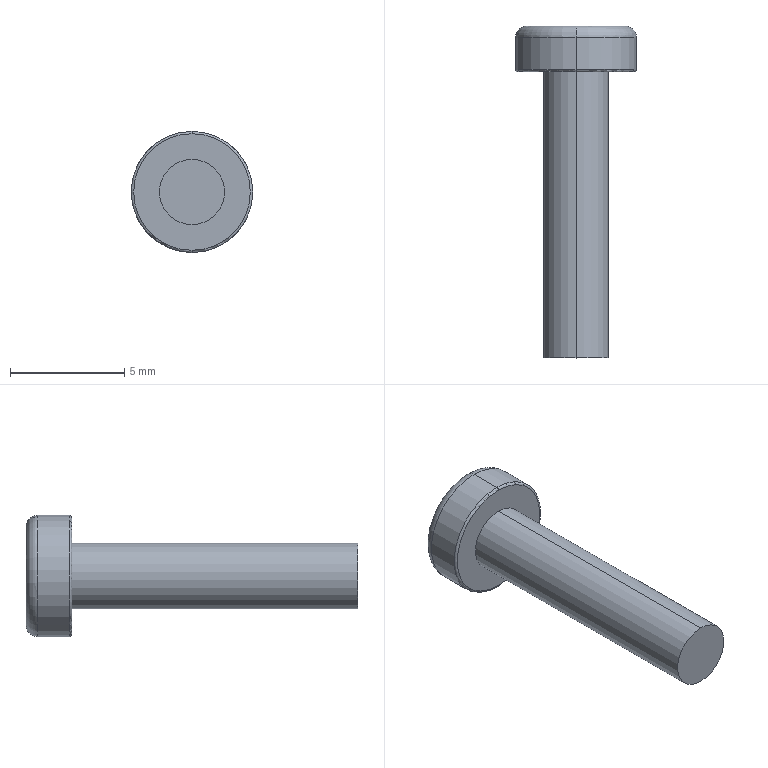Part | SolidWorks | features Fillet 2, ICE 2, Extrusion 1, Helix 1 | 1 solid | 24 faces | box 5.3 x 14.5 x 5.3 mm | volume 122.133 mm3 | plane 16 | torus 4 | cylinder 4 | commonest cylinder face diameters 2.86 x2 5.3 x2
STEP:
#1=CARTESIAN_POINT('',(0.,0.,-2.55));
#2=VERTEX_POINT('',#1);
#3=CARTESIAN_POINT('',(0.,0.,2.55));
#4=VERTEX_POINT('',#3);
#5=CARTESIAN_POINT('',(0.,0.,0.));
#6=DIRECTION('',(0.,-1.,0.));
#7=DIRECTION('',(0.,0.,1.));
#8=AXIS2_PLACEMENT_3D('',#5,#6,#7);
#9=CIRCLE('',#8,2.55);
#10=EDGE_CURVE('',#2,#4,#9,.T.);
#11=ORIENTED_EDGE('',*,*,#10,.F.);
#12=CARTESIAN_POINT('',(0.,0.1,-2.65));
#13=VERTEX_POINT('',#12);
#14=CARTESIAN_POINT('',(0.,0.1,-2.55));
#15=DIRECTION('',(1.,0.,0.));
#16=DIRECTION('',(0.,0.,-1.));
#17=AXIS2_PLACEMENT_3D('',#14,#15,#16);
#18=CIRCLE('',#17,0.1);
#19=EDGE_CURVE('',#2,#13,#18,.T.);
#20=ORIENTED_EDGE('',*,*,#19,.T.);
#21=CARTESIAN_POINT('',(0.,0.1,2.65));
#22=VERTEX_POINT('',#21);
#23=CARTESIAN_POINT('',(0.,0.1,0.));
#24=DIRECTION('',(0.,1.,0.));
#25=DIRECTION('',(0.,0.,1.));
#26=AXIS2_PLACEMENT_3D('',#23,#24,#25);
#27=CIRCLE('',#26,2.65);
#28=EDGE_CURVE('',#22,#13,#27,.T.);
#29=ORIENTED_EDGE('',*,*,#28,.F.);
#30=CARTESIAN_POINT('',(0.,0.1,2.55));
#31=DIRECTION('',(-1.,0.,0.));
#32=DIRECTION('',(0.,0.,1.));
#33=AXIS2_PLACEMENT_3D('',#30,#31,#32);
#34=CIRCLE('',#33,0.1);
#35=EDGE_CURVE('',#4,#22,#34,.T.);
#36=ORIENTED_EDGE('',*,*,#35,.F.);
#37=EDGE_LOOP('',(#11,#20,#29,#36));
#38=FACE_OUTER_BOUND('',#37,.T.);
#39=CARTESIAN_POINT('',(0.,0.1,0.));
#40=DIRECTION('',(0.,1.,0.));
#41=DIRECTION('',(0.,0.,1.));
#42=AXIS2_PLACEMENT_3D('',#39,#40,#41);
#43=TOROIDAL_SURFACE('',#42,2.55,0.1);
#44=ADVANCED_FACE('',(#38),#43,.T.);
#45=CARTESIAN_POINT('',(0.,1.5,-2.65));
#46=VERTEX_POINT('',#45);
#47=CARTESIAN_POINT('',(0.,1.5,2.65));
#48=VERTEX_POINT('',#47);
#49=CARTESIAN_POINT('',(0.,1.5,0.));
#50=DIRECTION('',(0.,-1.,0.));
#51=DIRECTION('',(0.,0.,1.));
#52=AXIS2_PLACEMENT_3D('',#49,#50,#51);
#53=CIRCLE('',#52,2.65);
#54=EDGE_CURVE('',#46,#48,#53,.T.);
#55=ORIENTED_EDGE('',*,*,#54,.F.);
#56=CARTESIAN_POINT('',(0.,2.,-2.15));
#57=VERTEX_POINT('',#56);
#58=CARTESIAN_POINT('',(0.,1.5,-2.15));
#59=DIRECTION('',(1.,0.,0.));
#60=DIRECTION('',(0.,0.,-1.));
#61=AXIS2_PLACEMENT_3D('',#58,#59,#60);
#62=CIRCLE('',#61,0.5);
#63=EDGE_CURVE('',#46,#57,#62,.T.);
#64=ORIENTED_EDGE('',*,*,#63,.T.);
#65=CARTESIAN_POINT('',(0.,2.,2.15));
#66=VERTEX_POINT('',#65);
#67=CARTESIAN_POINT('',(0.,2.,0.));
#68=DIRECTION('',(0.,1.,0.));
#69=DIRECTION('',(0.,0.,1.));
#70=AXIS2_PLACEMENT_3D('',#67,#68,#69);
#71=CIRCLE('',#70,2.15);
#72=EDGE_CURVE('',#66,#57,#71,.T.);
#73=ORIENTED_EDGE('',*,*,#72,.F.);
#74=CARTESIAN_POINT('',(0.,1.5,2.15));
#75=DIRECTION('',(-1.,0.,0.));
#76=DIRECTION('',(0.,0.,1.));
#77=AXIS2_PLACEMENT_3D('',#74,#75,#76);
#78=CIRCLE('',#77,0.5);
#79=EDGE_CURVE('',#48,#66,#78,.T.);
#80=ORIENTED_EDGE('',*,*,#79,.F.);
#81=EDGE_LOOP('',(#55,#64,#73,#80));
#82=FACE_OUTER_BOUND('',#81,.T.);
#83=CARTESIAN_POINT('',(0.,1.5,0.));
#84=DIRECTION('',(0.,1.,0.));
#85=DIRECTION('',(0.,0.,1.));
#86=AXIS2_PLACEMENT_3D('',#83,#84,#85);
#87=TOROIDAL_SURFACE('',#86,2.15,0.5);
#88=ADVANCED_FACE('',(#82),#87,.T.);
#89=CARTESIAN_POINT('',(0.,-12.5,-1.43));
#90=VERTEX_POINT('',#89);
#91=CARTESIAN_POINT('',(0.,-12.5,1.43));
#92=VERTEX_POINT('',#91);
#93=CARTESIAN_POINT('',(0.,-12.5,0.));
#94=DIRECTION('',(0.,-1.,0.));
#95=DIRECTION('',(0.,0.,-1.));
#96=AXIS2_PLACEMENT_3D('',#93,#94,#95);
#97=CIRCLE('',#96,1.43);
#98=EDGE_CURVE('',#90,#92,#97,.T.);
#99=ORIENTED_EDGE('',*,*,#98,.F.);
#100=CARTESIAN_POINT('',(0.,0.,-1.43));
#101=VERTEX_POINT('',#100);
#102=CARTESIAN_POINT('',(0.,-12.5,-1.43));
#103=DIRECTION('',(0.,1.,0.));
#104=VECTOR('',#103,1000.);
#105=LINE('',#102,#104);
#106=EDGE_CURVE('',#90,#101,#105,.T.);
#107=ORIENTED_EDGE('',*,*,#106,.T.);
#108=CARTESIAN_POINT('',(0.,0.,1.43));
#109=VERTEX_POINT('',#108);
#110=CARTESIAN_POINT('',(0.,0.,0.));
#111=DIRECTION('',(0.,-1.,0.));
#112=DIRECTION('',(0.,0.,1.));
#113=AXIS2_PLACEMENT_3D('',#110,#111,#112);
#114=CIRCLE('',#113,1.43);
#115=EDGE_CURVE('',#101,#109,#114,.T.);
#116=ORIENTED_EDGE('',*,*,#115,.T.);
#117=CARTESIAN_POINT('',(0.,-12.5,1.43));
#118=DIRECTION('',(0.,1.,0.));
#119=VECTOR('',#118,1000.);
#120=LINE('',#117,#119);
#121=EDGE_CURVE('',#92,#109,#120,.T.);
#122=ORIENTED_EDGE('',*,*,#121,.F.);
#123=EDGE_LOOP('',(#99,#107,#116,#122));
#124=FACE_OUTER_BOUND('',#123,.T.);
#125=CARTESIAN_POINT('',(0.,-12.5,0.));
#126=DIRECTION('',(0.,1.,0.));
#127=DIRECTION('',(0.,0.,1.));
#128=AXIS2_PLACEMENT_3D('',#125,#126,#127);
#129=CYLINDRICAL_SURFACE('',#128,1.43);
#130=ADVANCED_FACE('',(#124),#129,.T.);
#131=ORIENTED_EDGE('',*,*,#54,.T.);
#132=CARTESIAN_POINT('',(0.,2.,2.65));
#133=DIRECTION('',(0.,-1.,0.));
#134=VECTOR('',#133,1000.);
#135=LINE('',#132,#134);
#136=EDGE_CURVE('',#48,#22,#135,.T.);
#137=ORIENTED_EDGE('',*,*,#136,.T.);
#138=ORIENTED_EDGE('',*,*,#28,.T.);
#139=CARTESIAN_POINT('',(0.,2.,-2.65));
#140=DIRECTION('',(0.,-1.,0.));
#141=VECTOR('',#140,1000.);
#142=LINE('',#139,#141);
#143=EDGE_CURVE('',#46,#13,#142,.T.);
#144=ORIENTED_EDGE('',*,*,#143,.F.);
#145=EDGE_LOOP('',(#131,#137,#138,#144));
#146=FACE_OUTER_BOUND('',#145,.T.);
#147=CARTESIAN_POINT('',(0.,2.,0.));
#148=DIRECTION('',(0.,-1.,0.));
#149=DIRECTION('',(0.,0.,-1.));
#150=AXIS2_PLACEMENT_3D('',#147,#148,#149);
#151=CYLINDRICAL_SURFACE('',#150,2.65);
#152=ADVANCED_FACE('',(#146),#151,.T.);
#153=ORIENTED_EDGE('',*,*,#136,.F.);
#154=CARTESIAN_POINT('',(0.,1.5,0.));
#155=DIRECTION('',(0.,-1.,0.));
#156=DIRECTION('',(0.,0.,1.));
#157=AXIS2_PLACEMENT_3D('',#154,#155,#156);
#158=CIRCLE('',#157,2.65);
#159=EDGE_CURVE('',#48,#46,#158,.T.);
#160=ORIENTED_EDGE('',*,*,#159,.T.);
#161=ORIENTED_EDGE('',*,*,#143,.T.);
#162=CARTESIAN_POINT('',(0.,0.1,0.));
#163=DIRECTION('',(0.,1.,0.));
#164=DIRECTION('',(0.,0.,1.));
#165=AXIS2_PLACEMENT_3D('',#162,#163,#164);
#166=CIRCLE('',#165,2.65);
#167=EDGE_CURVE('',#13,#22,#166,.T.);
#168=ORIENTED_EDGE('',*,*,#167,.T.);
#169=EDGE_LOOP('',(#153,#160,#161,#168));
#170=FACE_OUTER_BOUND('',#169,.T.);
#171=CARTESIAN_POINT('',(0.,2.,0.));
#172=DIRECTION('',(0.,-1.,0.));
#173=DIRECTION('',(0.,0.,-1.));
#174=AXIS2_PLACEMENT_3D('',#171,#172,#173);
#175=CYLINDRICAL_SURFACE('',#174,2.65);
#176=ADVANCED_FACE('',(#170),#175,.T.);
#177=CARTESIAN_POINT('',(1.341,2.,0.3));
#178=VERTEX_POINT('',#177);
#179=CARTESIAN_POINT('',(1.341,2.,-0.3));
#180=VERTEX_POINT('',#179);
#181=CARTESIAN_POINT('',(1.341,2.,0.3));
#182=DIRECTION('',(0.,0.,-1.));
#183=VECTOR('',#182,1000.);
#184=LINE('',#181,#183);
#185=EDGE_CURVE('',#178,#180,#184,.T.);
#186=ORIENTED_EDGE('',*,*,#185,.F.);
#187=CARTESIAN_POINT('',(0.2966,2.,0.3));
#188=VERTEX_POINT('',#187);
#189=CARTESIAN_POINT('',(0.2966,2.,0.3));
#190=DIRECTION('',(1.,0.,0.));
#191=VECTOR('',#190,1000.);
#192=LINE('',#189,#191);
#193=EDGE_CURVE('',#188,#178,#192,.T.);
#194=ORIENTED_EDGE('',*,*,#193,.F.);
#195=CARTESIAN_POINT('',(0.2966,2.,1.336));
#196=VERTEX_POINT('',#195);
#197=CARTESIAN_POINT('',(0.2966,2.,1.336));
#198=DIRECTION('',(0.,0.,-1.));
#199=VECTOR('',#198,1000.);
#200=LINE('',#197,#199);
#201=EDGE_CURVE('',#196,#188,#200,.T.);
#202=ORIENTED_EDGE('',*,*,#201,.F.);
#203=CARTESIAN_POINT('',(-0.3034,2.,1.336));
#204=VERTEX_POINT('',#203);
#205=CARTESIAN_POINT('',(-0.3034,2.,1.336));
#206=DIRECTION('',(1.,0.,0.));
#207=VECTOR('',#206,1000.);
#208=LINE('',#205,#207);
#209=EDGE_CURVE('',#204,#196,#208,.T.);
#210=ORIENTED_EDGE('',*,*,#209,.F.);
#211=CARTESIAN_POINT('',(-0.3034,2.,0.3));
#212=VERTEX_POINT('',#211);
#213=CARTESIAN_POINT('',(-0.3034,2.,1.336));
#214=DIRECTION('',(0.,0.,1.));
#215=VECTOR('',#214,1000.);
#216=LINE('',#213,#215);
#217=EDGE_CURVE('',#212,#204,#216,.T.);
#218=ORIENTED_EDGE('',*,*,#217,.F.);
#219=CARTESIAN_POINT('',(-1.341,2.,0.3));
#220=VERTEX_POINT('',#219);
#221=CARTESIAN_POINT('',(-1.341,2.,0.3));
#222=DIRECTION('',(1.,0.,0.));
#223=VECTOR('',#222,1000.);
#224=LINE('',#221,#223);
#225=EDGE_CURVE('',#220,#212,#224,.T.);
#226=ORIENTED_EDGE('',*,*,#225,.F.);
#227=CARTESIAN_POINT('',(-1.341,2.,-0.3));
#228=VERTEX_POINT('',#227);
#229=CARTESIAN_POINT('',(-1.341,2.,0.3));
#230=DIRECTION('',(0.,0.,1.));
#231=VECTOR('',#230,1000.);
#232=LINE('',#229,#231);
#233=EDGE_CURVE('',#228,#220,#232,.T.);
#234=ORIENTED_EDGE('',*,*,#233,.F.);
#235=CARTESIAN_POINT('',(-0.3034,2.,-0.3));
#236=VERTEX_POINT('',#235);
#237=CARTESIAN_POINT('',(-1.341,2.,-0.3));
#238=DIRECTION('',(-1.,0.,0.));
#239=VECTOR('',#238,1000.);
#240=LINE('',#237,#239);
#241=EDGE_CURVE('',#236,#228,#240,.T.);
#242=ORIENTED_EDGE('',*,*,#241,.F.);
#243=CARTESIAN_POINT('',(-0.3034,2.,-1.336));
#244=VERTEX_POINT('',#243);
#245=CARTESIAN_POINT('',(-0.3034,2.,-0.3));
#246=DIRECTION('',(0.,0.,1.));
#247=VECTOR('',#246,1000.);
#248=LINE('',#245,#247);
#249=EDGE_CURVE('',#244,#236,#248,.T.);
#250=ORIENTED_EDGE('',*,*,#249,.F.);
#251=CARTESIAN_POINT('',(0.2966,2.,-1.336));
#252=VERTEX_POINT('',#251);
#253=CARTESIAN_POINT('',(-0.3034,2.,-1.336));
#254=DIRECTION('',(-1.,0.,0.));
#255=VECTOR('',#254,1000.);
#256=LINE('',#253,#255);
#257=EDGE_CURVE('',#252,#244,#256,.T.);
#258=ORIENTED_EDGE('',*,*,#257,.F.);
#259=CARTESIAN_POINT('',(0.2966,2.,-0.3));
#260=VERTEX_POINT('',#259);
#261=CARTESIAN_POINT('',(0.2966,2.,-0.3));
#262=DIRECTION('',(0.,0.,-1.));
#263=VECTOR('',#262,1000.);
#264=LINE('',#261,#263);
#265=EDGE_CURVE('',#260,#252,#264,.T.);
#266=ORIENTED_EDGE('',*,*,#265,.F.);
#267=CARTESIAN_POINT('',(0.2966,2.,-0.3));
#268=DIRECTION('',(-1.,0.,0.));
#269=VECTOR('',#268,1000.);
#270=LINE('',#267,#269);
#271=EDGE_CURVE('',#180,#260,#270,.T.);
#272=ORIENTED_EDGE('',*,*,#271,.F.);
#273=EDGE_LOOP('',(#186,#194,#202,#210,#218,#226,#234,#242,#250,#258,#266,#272));
#274=FACE_BOUND('',#273,.T.);
#275=ORIENTED_EDGE('',*,*,#72,.T.);
#276=CARTESIAN_POINT('',(0.,2.,0.));
#277=DIRECTION('',(0.,1.,0.));
#278=DIRECTION('',(0.,0.,1.));
#279=AXIS2_PLACEMENT_3D('',#276,#277,#278);
#280=CIRCLE('',#279,2.15);
#281=EDGE_CURVE('',#57,#66,#280,.T.);
#282=ORIENTED_EDGE('',*,*,#281,.T.);
#283=EDGE_LOOP('',(#275,#282));
#284=FACE_OUTER_BOUND('',#283,.T.);
#285=CARTESIAN_POINT('',(0.,2.,0.));
#286=DIRECTION('',(0.,1.,0.));
#287=DIRECTION('',(0.,0.,1.));
#288=AXIS2_PLACEMENT_3D('',#285,#286,#287);
#289=PLANE('',#288);
#290=ADVANCED_FACE('',(#274,#284),#289,.T.);
#291=CARTESIAN_POINT('',(0.,0.,0.));
#292=DIRECTION('',(0.,-1.,0.));
#293=DIRECTION('',(0.,0.,1.));
#294=AXIS2_PLACEMENT_3D('',#291,#292,#293);
#295=CIRCLE('',#294,2.55);
#296=EDGE_CURVE('',#4,#2,#295,.T.);
#297=ORIENTED_EDGE('',*,*,#296,.T.);
#298=ORIENTED_EDGE('',*,*,#10,.T.);
#299=EDGE_LOOP('',(#297,#298));
#300=FACE_OUTER_BOUND('',#299,.T.);
#301=CARTESIAN_POINT('',(0.,0.,0.));
#302=DIRECTION('',(0.,-1.,0.));
#303=DIRECTION('',(0.,0.,1.));
#304=AXIS2_PLACEMENT_3D('',#301,#302,#303);
#305=CIRCLE('',#304,1.43);
#306=EDGE_CURVE('',#109,#101,#305,.T.);
#307=ORIENTED_EDGE('',*,*,#306,.F.);
#308=ORIENTED_EDGE('',*,*,#115,.F.);
#309=EDGE_LOOP('',(#307,#308));
#310=FACE_BOUND('',#309,.T.);
#311=CARTESIAN_POINT('',(0.,0.,0.));
#312=DIRECTION('',(0.,1.,0.));
#313=DIRECTION('',(0.,0.,1.));
#314=AXIS2_PLACEMENT_3D('',#311,#312,#313);
#315=PLANE('',#314);
#316=ADVANCED_FACE('',(#300,#310),#315,.F.);
#317=ORIENTED_EDGE('',*,*,#106,.F.);
#318=CARTESIAN_POINT('',(0.,-12.5,0.));
#319=DIRECTION('',(0.,-1.,0.));
#320=DIRECTION('',(0.,0.,-1.));
#321=AXIS2_PLACEMENT_3D('',#318,#319,#320);
#322=CIRCLE('',#321,1.43);
#323=EDGE_CURVE('',#92,#90,#322,.T.);
#324=ORIENTED_EDGE('',*,*,#323,.F.);
#325=ORIENTED_EDGE('',*,*,#121,.T.);
#326=ORIENTED_EDGE('',*,*,#306,.T.);
#327=EDGE_LOOP('',(#317,#324,#325,#326));
#328=FACE_OUTER_BOUND('',#327,.T.);
#329=CARTESIAN_POINT('',(0.,-12.5,0.));
#330=DIRECTION('',(0.,1.,0.));
#331=DIRECTION('',(0.,0.,1.));
#332=AXIS2_PLACEMENT_3D('',#329,#330,#331);
#333=CYLINDRICAL_SURFACE('',#332,1.43);
#334=ADVANCED_FACE('',(#328),#333,.T.);
#335=ORIENTED_EDGE('',*,*,#323,.T.);
#336=ORIENTED_EDGE('',*,*,#98,.T.);
#337=EDGE_LOOP('',(#335,#336));
#338=FACE_OUTER_BOUND('',#337,.T.);
#339=CARTESIAN_POINT('',(0.,-12.5,0.));
#340=DIRECTION('',(0.,-1.,0.));
#341=DIRECTION('',(0.,0.,-1.));
#342=AXIS2_PLACEMENT_3D('',#339,#340,#341);
#343=PLANE('',#342);
#344=ADVANCED_FACE('',(#338),#343,.T.);
#345=ORIENTED_EDGE('',*,*,#63,.F.);
#346=ORIENTED_EDGE('',*,*,#159,.F.);
#347=ORIENTED_EDGE('',*,*,#79,.T.);
#348=ORIENTED_EDGE('',*,*,#281,.F.);
#349=EDGE_LOOP('',(#345,#346,#347,#348));
#350=FACE_OUTER_BOUND('',#349,.T.);
#351=CARTESIAN_POINT('',(0.,1.5,0.));
#352=DIRECTION('',(0.,1.,0.));
#353=DIRECTION('',(0.,0.,1.));
#354=AXIS2_PLACEMENT_3D('',#351,#352,#353);
#355=TOROIDAL_SURFACE('',#354,2.15,0.5);
#356=ADVANCED_FACE('',(#350),#355,.T.);
#357=ORIENTED_EDGE('',*,*,#19,.F.);
#358=ORIENTED_EDGE('',*,*,#296,.F.);
#359=ORIENTED_EDGE('',*,*,#35,.T.);
#360=ORIENTED_EDGE('',*,*,#167,.F.);
#361=EDGE_LOOP('',(#357,#358,#359,#360));
#362=FACE_OUTER_BOUND('',#361,.T.);
#363=CARTESIAN_POINT('',(0.,0.1,0.));
#364=DIRECTION('',(0.,1.,0.));
#365=DIRECTION('',(0.,0.,1.));
#366=AXIS2_PLACEMENT_3D('',#363,#364,#365);
#367=TOROIDAL_SURFACE('',#366,2.55,0.1);
#368=ADVANCED_FACE('',(#362),#367,.T.);
#369=ORIENTED_EDGE('',*,*,#185,.T.);
#370=CARTESIAN_POINT('',(1.332,1.5,-0.2913));
#371=VERTEX_POINT('',#370);
#372=CARTESIAN_POINT('',(1.34,1.99,-0.2998));
#373=DIRECTION('',(0.01745,0.9997,-0.01745));
#374=VECTOR('',#373,1000.);
#375=LINE('',#372,#374);
#376=EDGE_CURVE('',#371,#180,#375,.T.);
#377=ORIENTED_EDGE('',*,*,#376,.F.);
#378=CARTESIAN_POINT('',(1.332,1.5,0.2913));
#379=VERTEX_POINT('',#378);
#380=CARTESIAN_POINT('',(1.332,1.5,0.3));
#381=DIRECTION('',(0.,0.,-1.));
#382=VECTOR('',#381,1000.);
#383=LINE('',#380,#382);
#384=EDGE_CURVE('',#379,#371,#383,.T.);
#385=ORIENTED_EDGE('',*,*,#384,.F.);
#386=CARTESIAN_POINT('',(1.34,1.982,0.2997));
#387=DIRECTION('',(0.01745,0.9997,0.01745));
#388=VECTOR('',#387,1000.);
#389=LINE('',#386,#388);
#390=EDGE_CURVE('',#379,#178,#389,.T.);
#391=ORIENTED_EDGE('',*,*,#390,.T.);
#392=EDGE_LOOP('',(#369,#377,#385,#391));
#393=FACE_OUTER_BOUND('',#392,.T.);
#394=CARTESIAN_POINT('',(1.341,2.,0.3));
#395=DIRECTION('',(0.9998,-0.01745,0.));
#396=DIRECTION('',(0.01745,0.9998,0.));
#397=AXIS2_PLACEMENT_3D('',#394,#395,#396);
#398=PLANE('',#397);
#399=ADVANCED_FACE('',(#393),#398,.F.);
#400=ORIENTED_EDGE('',*,*,#193,.T.);
#401=ORIENTED_EDGE('',*,*,#390,.F.);
#402=CARTESIAN_POINT('',(0.2878,1.5,0.2913));
#403=VERTEX_POINT('',#402);
#404=CARTESIAN_POINT('',(0.2966,1.5,0.2913));
#405=DIRECTION('',(1.,0.,0.));
#406=VECTOR('',#405,1000.);
#407=LINE('',#404,#406);
#408=EDGE_CURVE('',#403,#379,#407,.T.);
#409=ORIENTED_EDGE('',*,*,#408,.F.);
#410=CARTESIAN_POINT('',(0.2966,2.,0.3));
#411=DIRECTION('',(0.01745,0.9997,0.01745));
#412=VECTOR('',#411,1000.);
#413=LINE('',#410,#412);
#414=EDGE_CURVE('',#403,#188,#413,.T.);
#415=ORIENTED_EDGE('',*,*,#414,.T.);
#416=EDGE_LOOP('',(#400,#401,#409,#415));
#417=FACE_OUTER_BOUND('',#416,.T.);
#418=CARTESIAN_POINT('',(0.2966,2.,0.3));
#419=DIRECTION('',(0.,-0.01745,0.9998));
#420=DIRECTION('',(0.,-0.9998,-0.01745));
#421=AXIS2_PLACEMENT_3D('',#418,#419,#420);
#422=PLANE('',#421);
#423=ADVANCED_FACE('',(#417),#422,.F.);
#424=ORIENTED_EDGE('',*,*,#201,.T.);
#425=ORIENTED_EDGE('',*,*,#414,.F.);
#426=CARTESIAN_POINT('',(0.2878,1.5,1.327));
#427=VERTEX_POINT('',#426);
#428=CARTESIAN_POINT('',(0.2878,1.5,1.336));
#429=DIRECTION('',(0.,0.,-1.));
#430=VECTOR('',#429,1000.);
#431=LINE('',#428,#430);
#432=EDGE_CURVE('',#427,#403,#431,.T.);
#433=ORIENTED_EDGE('',*,*,#432,.F.);
#434=CARTESIAN_POINT('',(0.2964,1.99,1.336));
#435=DIRECTION('',(0.01745,0.9997,0.01745));
#436=VECTOR('',#435,1000.);
#437=LINE('',#434,#436);
#438=EDGE_CURVE('',#427,#196,#437,.T.);
#439=ORIENTED_EDGE('',*,*,#438,.T.);
#440=EDGE_LOOP('',(#424,#425,#433,#439));
#441=FACE_OUTER_BOUND('',#440,.T.);
#442=CARTESIAN_POINT('',(0.2966,2.,1.336));
#443=DIRECTION('',(0.9998,-0.01745,0.));
#444=DIRECTION('',(0.01745,0.9998,0.));
#445=AXIS2_PLACEMENT_3D('',#442,#443,#444);
#446=PLANE('',#445);
#447=ADVANCED_FACE('',(#441),#446,.F.);
#448=ORIENTED_EDGE('',*,*,#209,.T.);
#449=ORIENTED_EDGE('',*,*,#438,.F.);
#450=CARTESIAN_POINT('',(-0.2947,1.5,1.327));
#451=VERTEX_POINT('',#450);
#452=CARTESIAN_POINT('',(-0.3034,1.5,1.327));
#453=DIRECTION('',(1.,0.,0.));
#454=VECTOR('',#453,1000.);
#455=LINE('',#452,#454);
#456=EDGE_CURVE('',#451,#427,#455,.T.);
#457=ORIENTED_EDGE('',*,*,#456,.F.);
#458=CARTESIAN_POINT('',(-0.3034,2.,1.336));
#459=DIRECTION('',(-0.01745,0.9997,0.01745));
#460=VECTOR('',#459,1000.);
#461=LINE('',#458,#460);
#462=EDGE_CURVE('',#451,#204,#461,.T.);
#463=ORIENTED_EDGE('',*,*,#462,.T.);
#464=EDGE_LOOP('',(#448,#449,#457,#463));
#465=FACE_OUTER_BOUND('',#464,.T.);
#466=CARTESIAN_POINT('',(-0.3034,2.,1.336));
#467=DIRECTION('',(0.,-0.01745,0.9998));
#468=DIRECTION('',(0.,-0.9998,-0.01745));
#469=AXIS2_PLACEMENT_3D('',#466,#467,#468);
#470=PLANE('',#469);
#471=ADVANCED_FACE('',(#465),#470,.F.);
#472=ORIENTED_EDGE('',*,*,#217,.T.);
#473=ORIENTED_EDGE('',*,*,#462,.F.);
#474=CARTESIAN_POINT('',(-0.2947,1.5,0.2913));
#475=VERTEX_POINT('',#474);
#476=CARTESIAN_POINT('',(-0.2947,1.5,1.336));
#477=DIRECTION('',(0.,0.,1.));
#478=VECTOR('',#477,1000.);
#479=LINE('',#476,#478);
#480=EDGE_CURVE('',#475,#451,#479,.T.);
#481=ORIENTED_EDGE('',*,*,#480,.F.);
#482=CARTESIAN_POINT('',(-0.3037,2.018,0.3003));
#483=DIRECTION('',(-0.01745,0.9997,0.01745));
#484=VECTOR('',#483,1000.);
#485=LINE('',#482,#484);
#486=EDGE_CURVE('',#475,#212,#485,.T.);
#487=ORIENTED_EDGE('',*,*,#486,.T.);
#488=EDGE_LOOP('',(#472,#473,#481,#487));
#489=FACE_OUTER_BOUND('',#488,.T.);
#490=CARTESIAN_POINT('',(-0.3034,2.,1.336));
#491=DIRECTION('',(-0.9998,-0.01745,0.));
#492=DIRECTION('',(0.01745,-0.9998,0.));
#493=AXIS2_PLACEMENT_3D('',#490,#491,#492);
#494=PLANE('',#493);
#495=ADVANCED_FACE('',(#489),#494,.F.);
#496=ORIENTED_EDGE('',*,*,#225,.T.);
#497=ORIENTED_EDGE('',*,*,#486,.F.);
#498=CARTESIAN_POINT('',(-1.332,1.5,0.2913));
#499=VERTEX_POINT('',#498);
#500=CARTESIAN_POINT('',(-1.341,1.5,0.2913));
#501=DIRECTION('',(1.,0.,0.));
#502=VECTOR('',#501,1000.);
#503=LINE('',#500,#502);
#504=EDGE_CURVE('',#499,#475,#503,.T.);
#505=ORIENTED_EDGE('',*,*,#504,.F.);
#506=CARTESIAN_POINT('',(-1.341,2.,0.3));
#507=DIRECTION('',(-0.01745,0.9997,0.01745));
#508=VECTOR('',#507,1000.);
#509=LINE('',#506,#508);
#510=EDGE_CURVE('',#499,#220,#509,.T.);
#511=ORIENTED_EDGE('',*,*,#510,.T.);
#512=EDGE_LOOP('',(#496,#497,#505,#511));
#513=FACE_OUTER_BOUND('',#512,.T.);
#514=CARTESIAN_POINT('',(-1.341,2.,0.3));
#515=DIRECTION('',(0.,-0.01745,0.9998));
#516=DIRECTION('',(0.,-0.9998,-0.01745));
#517=AXIS2_PLACEMENT_3D('',#514,#515,#516);
#518=PLANE('',#517);
#519=ADVANCED_FACE('',(#513),#518,.F.);
#520=ORIENTED_EDGE('',*,*,#233,.T.);
#521=ORIENTED_EDGE('',*,*,#510,.F.);
#522=CARTESIAN_POINT('',(-1.332,1.5,-0.2913));
#523=VERTEX_POINT('',#522);
#524=CARTESIAN_POINT('',(-1.332,1.5,0.3));
#525=DIRECTION('',(0.,0.,1.));
#526=VECTOR('',#525,1000.);
#527=LINE('',#524,#526);
#528=EDGE_CURVE('',#523,#499,#527,.T.);
#529=ORIENTED_EDGE('',*,*,#528,.F.);
#530=CARTESIAN_POINT('',(-1.341,2.,-0.3));
#531=DIRECTION('',(-0.01745,0.9997,-0.01745));
#532=VECTOR('',#531,1000.);
#533=LINE('',#530,#532);
#534=EDGE_CURVE('',#523,#228,#533,.T.);
#535=ORIENTED_EDGE('',*,*,#534,.T.);
#536=EDGE_LOOP('',(#520,#521,#529,#535));
#537=FACE_OUTER_BOUND('',#536,.T.);
#538=CARTESIAN_POINT('',(-1.341,2.,0.3));
#539=DIRECTION('',(-0.9998,-0.01745,0.));
#540=DIRECTION('',(0.01745,-0.9998,0.));
#541=AXIS2_PLACEMENT_3D('',#538,#539,#540);
#542=PLANE('',#541);
#543=ADVANCED_FACE('',(#537),#542,.F.);
#544=ORIENTED_EDGE('',*,*,#241,.T.);
#545=ORIENTED_EDGE('',*,*,#534,.F.);
#546=CARTESIAN_POINT('',(-0.2947,1.5,-0.2913));
#547=VERTEX_POINT('',#546);
#548=CARTESIAN_POINT('',(-1.341,1.5,-0.2913));
#549=DIRECTION('',(-1.,0.,0.));
#550=VECTOR('',#549,1000.);
#551=LINE('',#548,#550);
#552=EDGE_CURVE('',#547,#523,#551,.T.);
#553=ORIENTED_EDGE('',*,*,#552,.F.);
#554=CARTESIAN_POINT('',(-0.3037,2.018,-0.3003));
#555=DIRECTION('',(-0.01745,0.9997,-0.01745));
#556=VECTOR('',#555,1000.);
#557=LINE('',#554,#556);
#558=EDGE_CURVE('',#547,#236,#557,.T.);
#559=ORIENTED_EDGE('',*,*,#558,.T.);
#560=EDGE_LOOP('',(#544,#545,#553,#559));
#561=FACE_OUTER_BOUND('',#560,.T.);
#562=CARTESIAN_POINT('',(-1.341,2.,-0.3));
#563=DIRECTION('',(0.,-0.01745,-0.9998));
#564=DIRECTION('',(0.,0.9998,-0.01745));
#565=AXIS2_PLACEMENT_3D('',#562,#563,#564);
#566=PLANE('',#565);
#567=ADVANCED_FACE('',(#561),#566,.F.);
#568=ORIENTED_EDGE('',*,*,#249,.T.);
#569=ORIENTED_EDGE('',*,*,#558,.F.);
#570=CARTESIAN_POINT('',(-0.2947,1.5,-1.327));
#571=VERTEX_POINT('',#570);
#572=CARTESIAN_POINT('',(-0.2947,1.5,-0.3));
#573=DIRECTION('',(0.,0.,1.));
#574=VECTOR('',#573,1000.);
#575=LINE('',#572,#574);
#576=EDGE_CURVE('',#571,#547,#575,.T.);
#577=ORIENTED_EDGE('',*,*,#576,.F.);
#578=CARTESIAN_POINT('',(-0.3034,2.,-1.336));
#579=DIRECTION('',(-0.01745,0.9997,-0.01745));
#580=VECTOR('',#579,1000.);
#581=LINE('',#578,#580);
#582=EDGE_CURVE('',#571,#244,#581,.T.);
#583=ORIENTED_EDGE('',*,*,#582,.T.);
#584=EDGE_LOOP('',(#568,#569,#577,#583));
#585=FACE_OUTER_BOUND('',#584,.T.);
#586=CARTESIAN_POINT('',(-0.3034,2.,-0.3));
#587=DIRECTION('',(-0.9998,-0.01745,0.));
#588=DIRECTION('',(0.01745,-0.9998,0.));
#589=AXIS2_PLACEMENT_3D('',#586,#587,#588);
#590=PLANE('',#589);
#591=ADVANCED_FACE('',(#585),#590,.F.);
#592=ORIENTED_EDGE('',*,*,#257,.T.);
#593=ORIENTED_EDGE('',*,*,#582,.F.);
#594=CARTESIAN_POINT('',(0.2878,1.5,-1.327));
#595=VERTEX_POINT('',#594);
#596=CARTESIAN_POINT('',(-0.3034,1.5,-1.327));
#597=DIRECTION('',(-1.,0.,0.));
#598=VECTOR('',#597,1000.);
#599=LINE('',#596,#598);
#600=EDGE_CURVE('',#595,#571,#599,.T.);
#601=ORIENTED_EDGE('',*,*,#600,.F.);
#602=CARTESIAN_POINT('',(0.2963,1.982,-1.336));
#603=DIRECTION('',(0.01745,0.9997,-0.01745));
#604=VECTOR('',#603,1000.);
#605=LINE('',#602,#604);
#606=EDGE_CURVE('',#595,#252,#605,.T.);
#607=ORIENTED_EDGE('',*,*,#606,.T.);
#608=EDGE_LOOP('',(#592,#593,#601,#607));
#609=FACE_OUTER_BOUND('',#608,.T.);
#610=CARTESIAN_POINT('',(-0.3034,2.,-1.336));
#611=DIRECTION('',(0.,-0.01745,-0.9998));
#612=DIRECTION('',(0.,0.9998,-0.01745));
#613=AXIS2_PLACEMENT_3D('',#610,#611,#612);
#614=PLANE('',#613);
#615=ADVANCED_FACE('',(#609),#614,.F.);
#616=ORIENTED_EDGE('',*,*,#265,.T.);
#617=ORIENTED_EDGE('',*,*,#606,.F.);
#618=CARTESIAN_POINT('',(0.2878,1.5,-0.2913));
#619=VERTEX_POINT('',#618);
#620=CARTESIAN_POINT('',(0.2878,1.5,-0.3));
#621=DIRECTION('',(0.,0.,-1.));
#622=VECTOR('',#621,1000.);
#623=LINE('',#620,#622);
#624=EDGE_CURVE('',#619,#595,#623,.T.);
#625=ORIENTED_EDGE('',*,*,#624,.F.);
#626=CARTESIAN_POINT('',(0.2966,2.,-0.3));
#627=DIRECTION('',(0.01745,0.9997,-0.01745));
#628=VECTOR('',#627,1000.);
#629=LINE('',#626,#628);
#630=EDGE_CURVE('',#619,#260,#629,.T.);
#631=ORIENTED_EDGE('',*,*,#630,.T.);
#632=EDGE_LOOP('',(#616,#617,#625,#631));
#633=FACE_OUTER_BOUND('',#632,.T.);
#634=CARTESIAN_POINT('',(0.2966,2.,-0.3));
#635=DIRECTION('',(0.9998,-0.01745,0.));
#636=DIRECTION('',(0.01745,0.9998,0.));
#637=AXIS2_PLACEMENT_3D('',#634,#635,#636);
#638=PLANE('',#637);
#639=ADVANCED_FACE('',(#633),#638,.F.);
#640=ORIENTED_EDGE('',*,*,#271,.T.);
#641=ORIENTED_EDGE('',*,*,#630,.F.);
#642=CARTESIAN_POINT('',(0.2966,1.5,-0.2913));
#643=DIRECTION('',(-1.,0.,0.));
#644=VECTOR('',#643,1000.);
#645=LINE('',#642,#644);
#646=EDGE_CURVE('',#371,#619,#645,.T.);
#647=ORIENTED_EDGE('',*,*,#646,.F.);
#648=ORIENTED_EDGE('',*,*,#376,.T.);
#649=EDGE_LOOP('',(#640,#641,#647,#648));
#650=FACE_OUTER_BOUND('',#649,.T.);
#651=CARTESIAN_POINT('',(0.2966,2.,-0.3));
#652=DIRECTION('',(0.,-0.01745,-0.9998));
#653=DIRECTION('',(0.,0.9998,-0.01745));
#654=AXIS2_PLACEMENT_3D('',#651,#652,#653);
#655=PLANE('',#654);
#656=ADVANCED_FACE('',(#650),#655,.F.);
#657=ORIENTED_EDGE('',*,*,#384,.T.);
#658=ORIENTED_EDGE('',*,*,#646,.T.);
#659=ORIENTED_EDGE('',*,*,#624,.T.);
#660=ORIENTED_EDGE('',*,*,#600,.T.);
#661=ORIENTED_EDGE('',*,*,#576,.T.);
#662=ORIENTED_EDGE('',*,*,#552,.T.);
#663=ORIENTED_EDGE('',*,*,#528,.T.);
#664=ORIENTED_EDGE('',*,*,#504,.T.);
#665=ORIENTED_EDGE('',*,*,#480,.T.);
#666=ORIENTED_EDGE('',*,*,#456,.T.);
#667=ORIENTED_EDGE('',*,*,#432,.T.);
#668=ORIENTED_EDGE('',*,*,#408,.T.);
#669=EDGE_LOOP('',(#657,#658,#659,#660,#661,#662,#663,#664,#665,#666,#667,#668));
#670=FACE_OUTER_BOUND('',#669,.T.);
#671=CARTESIAN_POINT('',(0.,1.5,0.));
#672=DIRECTION('',(0.,-1.,0.));
#673=DIRECTION('',(0.,0.,-1.));
#674=AXIS2_PLACEMENT_3D('',#671,#672,#673);
#675=PLANE('',#674);
#676=ADVANCED_FACE('',(#670),#675,.F.);
#677=CLOSED_SHELL('',(#44,#88,#130,#152,#176,#290,#316,#334,#344,#356,#368,#399,#423,#447,#471,#495,#519,#543,#567,#591,#615,#639,#656,#676));
#678=MANIFOLD_SOLID_BREP('',#677);
#679=CARTESIAN_POINT('',(0.,0.,0.));
#680=DIRECTION('',(0.,0.,1.));
#681=DIRECTION('',(1.,0.,0.));
#682=AXIS2_PLACEMENT_3D('',#679,#680,#681);
#683=(LENGTH_UNIT()NAMED_UNIT(*)SI_UNIT(.MILLI.,.METRE.));
#684=UNCERTAINTY_MEASURE_WITH_UNIT(LENGTH_MEASURE(0.00001),#683,'','');
#685=(NAMED_UNIT(*)PLANE_ANGLE_UNIT()SI_UNIT($,.RADIAN.));
#686=(NAMED_UNIT(*)SI_UNIT($,.STERADIAN.)SOLID_ANGLE_UNIT());
#687=(GEOMETRIC_REPRESENTATION_CONTEXT(3)GLOBAL_UNCERTAINTY_ASSIGNED_CONTEXT((#684))GLOBAL_UNIT_ASSIGNED_CONTEXT((#683,#685,#686))REPRESENTATION_CONTEXT('',''));
#688=ADVANCED_BREP_SHAPE_REPRESENTATION('',(#678,#682),#687);